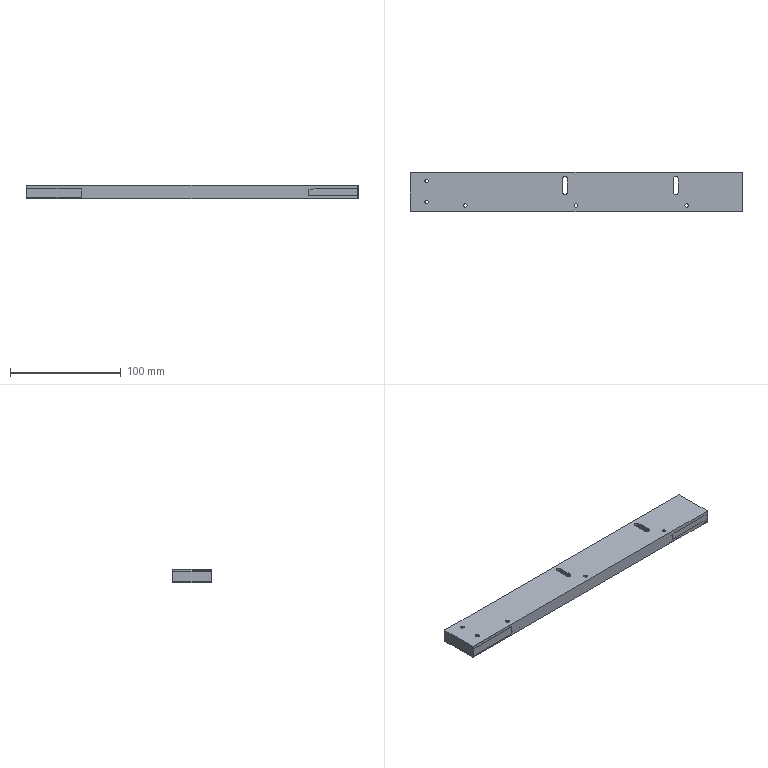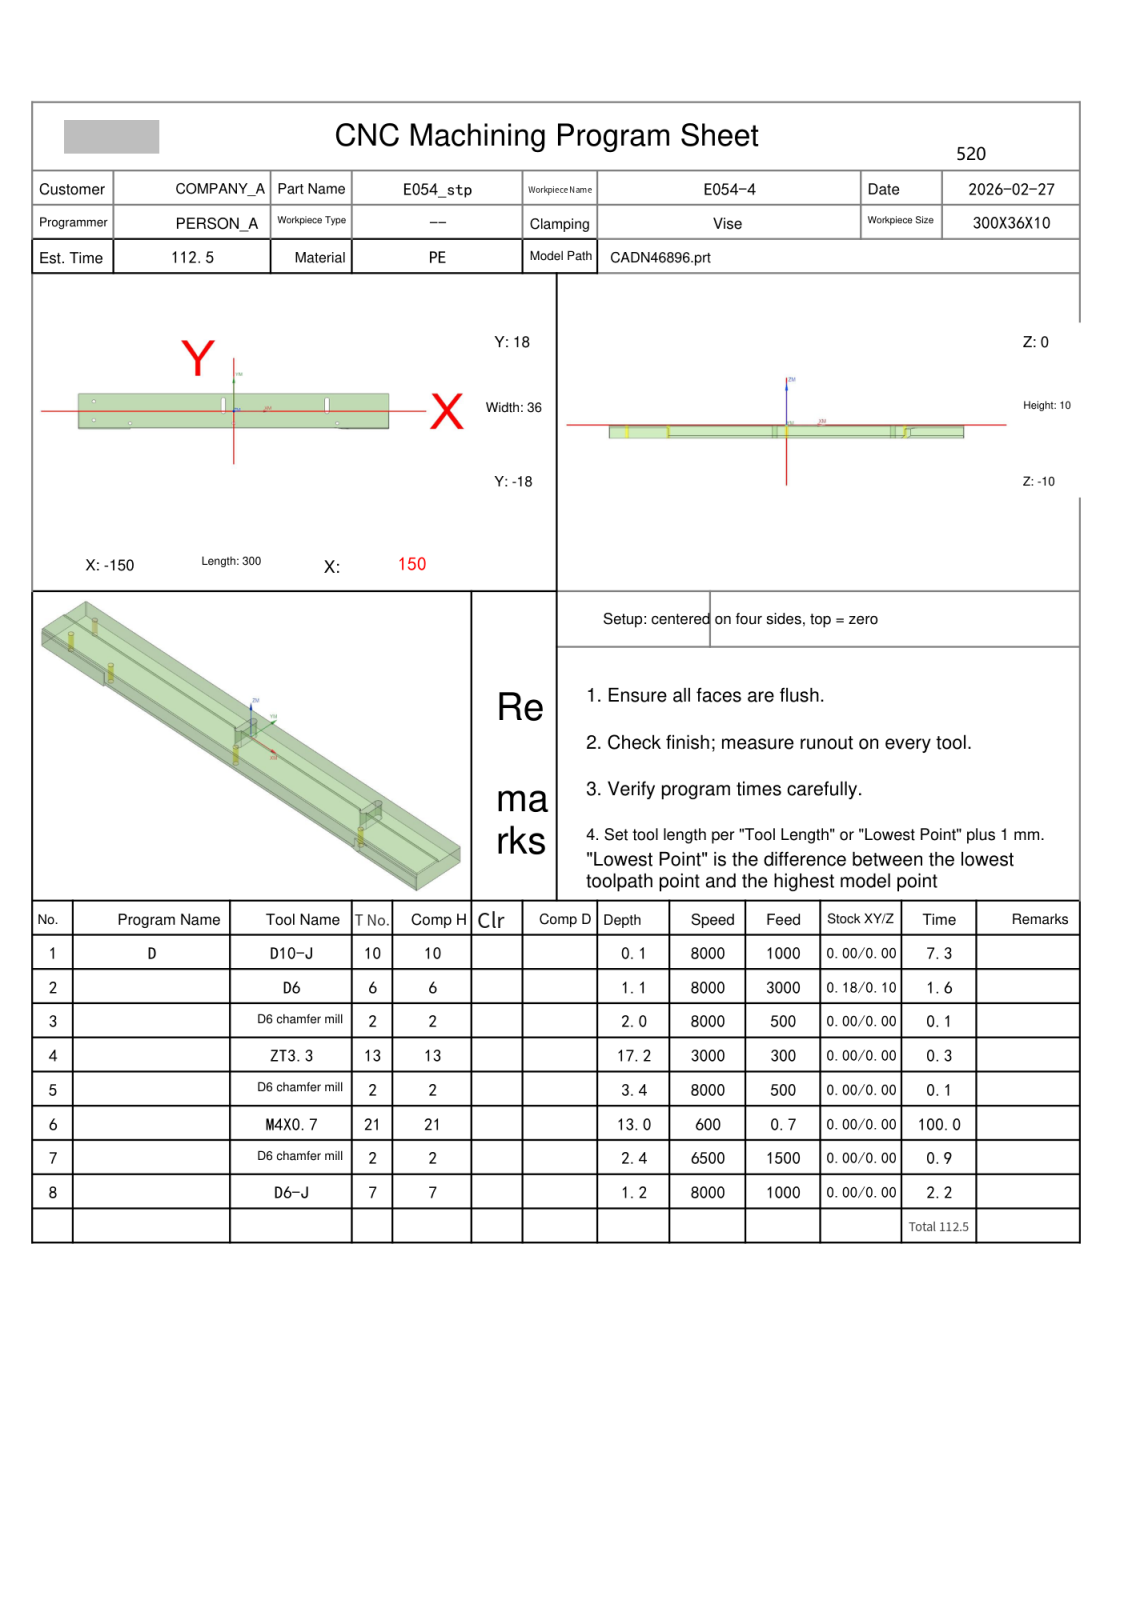NC program | NX | posted by the shop | part box 300 x 36 x 12 mm
Whole program:
%
O0001
(Machine time: 206.88 MIN)
(===Total Tool:6===)
(T10=D10-J  D=10.  R=0.   D-  H10 Z=0.    )
(T6=D6      D=6.   R=0.   D-  H06 Z=-1.1  )
(T2=D6 chamfer mill   D=6.   R=0.   D-  H02 Z=-3.37 )
(T13=ZT3.3  D=3.3  DR_a=118 D-  H13 Z=-17.2 )
(T21=M4X0.7 D=3.3  DR_a=180 D-  H21 Z=-13.  )
(T7=D6-J    D=6.   R=0.   D7  H07 Z=-1.2  )
G80 G90 G17 G49 G40
G91 G28 Z0
M01
N1 T10 M06
(D10-J  D=10. R=0. H=10 ce=0.00 di=0.10)
G00 G90 G54 X133.111 Y35. M03 S8000
G43 H10 Z50.
M08
Z2.55
G01 Z.55 F1000.
X145.111 Y23.
X155. Y13.111
Y3.222
X135.222 Y23.
X125.333
X155. Y-6.667
Y-16.556
X115.444 Y23.
X105.556
X151.556 Y-23.
X141.667
X95.667 Y23.
X85.778
X131.778 Y-23.
X121.889
X75.889 Y23.
X66.
X112. Y-23.
X102.111
X56.111 Y23.
X46.222
X92.222 Y-23.
X82.333
X36.333 Y23.
X26.444
X72.444 Y-23.
X62.556
X16.556 Y23.
X6.667
X52.667 Y-23.
X42.778
X-3.222 Y23.
X-13.111
X32.889 Y-23.
X23.
X-23. Y23.
X-32.889
X13.111 Y-23.
X3.222
X-42.778 Y23.
X-52.667
X-6.667 Y-23.
X-16.556
X-62.556 Y23.
X-72.444
X-26.444 Y-23.
X-36.333
X-82.333 Y23.
X-92.222
X-46.222 Y-23.
X-56.111
X-102.111 Y23.
X-112.
X-66. Y-23.
X-75.889
X-121.889 Y23.
X-131.778
X-85.778 Y-23.
X-95.667
X-141.667 Y23.
X-151.556
X-105.556 Y-23.
X-115.444
X-155. Y16.556
Y6.667
X-125.333 Y-23.
X-135.222
X-155. Y-3.222
Y-13.111
X-145.111 Y-23.
X-133.111 Y-35.
Z2.55
G00 Z4.
X167. Y1.111
Z2.1
G01 Z.1
X155. Y13.111
X145.111 Y23.
X135.222
X155. Y3.222
Y-6.667
X125.333 Y23.
X115.444
X155. Y-16.556
Y-23.
X151.556
X105.556 Y23.
X95.667
X141.667 Y-23.
X131.778
X85.778 Y23.
X75.889
X121.889 Y-23.
X112.
X66. Y23.
X56.111
X102.111 Y-23.
X92.222
X46.222 Y23.
X36.333
X82.333 Y-23.
X72.444
X26.444 Y23.
X16.556
X62.556 Y-23.
X52.667
X6.667 Y23.
X-3.222
X42.778 Y-23.
X32.889
X-13.111 Y23.
X-23.
X23. Y-23.
X13.111
X-32.889 Y23.
X-42.778
X3.222 Y-23.
X-6.667
X-52.667 Y23.
X-62.556
X-16.556 Y-23.
X-26.444
X-72.444 Y23.
X-82.333
X-36.333 Y-23.
X-46.222
X-92.222 Y23.
X-102.111
X-56.111 Y-23.
X-66.
X-112. Y23.
X-121.889
X-75.889 Y-23.
X-85.778
X-131.778 Y23.
X-141.667
X-95.667 Y-23.
X-105.556
X-151.556 Y23.
X-155.
Y16.556
X-115.444 Y-23.
X-125.333
X-155. Y6.667
Y-3.222
X-135.222 Y-23.
X-145.111
X-155. Y-13.111
X-167. Y-1.111
Z2.1
G00 Z50.
G00 G90 X133.111 Y35. M03 S8000
Z50.
Z2.
G01 Z0.0 F1000.
X145.111 Y23.
X155. Y13.111
Y3.222
X135.222 Y23.
X125.333
X155. Y-6.667
Y-16.556
X115.444 Y23.
X105.556
X151.556 Y-23.
X141.667
X95.667 Y23.
X85.778
X131.778 Y-23.
X121.889
X75.889 Y23.
X66.
X112. Y-23.
X102.111
X56.111 Y23.
X46.222
X92.222 Y-23.
X82.333
X36.333 Y23.
X26.444
X72.444 Y-23.
X62.556
X16.556 Y23.
X6.667
X52.667 Y-23.
X42.778
X-3.222 Y23.
X-13.111
X32.889 Y-23.
X23.
X-23. Y23.
X-32.889
X13.111 Y-23.
X3.222
X-42.778 Y23.
X-52.667
X-6.667 Y-23.
X-16.556
X-62.556 Y23.
X-72.444
X-26.444 Y-23.
X-36.333
X-82.333 Y23.
X-92.222
X-46.222 Y-23.
X-56.111
X-102.111 Y23.
X-112.
X-66. Y-23.
X-75.889
X-121.889 Y23.
X-131.778
X-85.778 Y-23.
X-95.667
X-141.667 Y23.
X-151.556
X-105.556 Y-23.
X-115.444
X-155. Y16.556
Y6.667
X-125.333 Y-23.
X-135.222
X-155. Y-3.222
Y-13.111
X-145.111 Y-23.
X-133.111 Y-35.
Z2.
G00 Z50.
G91 G28 Z0.0
M05
M09
G91 G28 Z0.0
M01
N2 T06 M06
(D6  D=6. R=0. H=06 ce=0.18 di=0.10)
G00 G90 G54 X-155.845 Y19.68 M03 S8000
G43 H06 Z11.
M08
Z1.133
G01 Z-.367 F3000.
X-151.978
X151.73
G02 X152.153 Y19.505 I-.001 J-.6
G01 X152.764 Y18.893
G02 X152.94 Y18.469 I-.424 J-.424
G01 Y17.279
G02 X152.341 Y16.68 I-.6 J.001
G01 X-152.341
G03 X-152.94 Y16.081 I.001 J-.6
G01 Y12.779
G03 X-152.341 Y12.18 I.6 J.001
G01 X152.341
G02 X152.94 Y11.581 I-.001 J-.6
G01 Y8.279
G02 X152.341 Y7.68 I-.6 J.001
G01 X-152.427
G03 X-153.019 Y7.173 I.001 J-.6
G01 X-153.533 Y3.872
X-153.54 Y3.78
G03 X-152.94 Y3.18 I.6 J0.0
G01 X152.94
X156.047
Z1.133
G00 X-155.845 Y19.68
Z.767
G01 Z-.733
X-151.978
X151.73
G02 X152.153 Y19.505 I-.001 J-.6
G01 X152.764 Y18.893
G02 X152.94 Y18.469 I-.424 J-.424
G01 Y17.279
G02 X152.341 Y16.68 I-.6 J.001
G01 X-152.341
G03 X-152.94 Y16.081 I.001 J-.6
G01 Y12.779
G03 X-152.341 Y12.18 I.6 J.001
G01 X152.341
G02 X152.94 Y11.581 I-.001 J-.6
G01 Y8.279
G02 X152.341 Y7.68 I-.6 J.001
G01 X-152.427
G03 X-153.019 Y7.173 I.001 J-.6
G01 X-153.533 Y3.872
X-153.54 Y3.78
G03 X-152.94 Y3.18 I.6 J0.0
G01 X152.94
X156.18
Z.767
G00 X-155.845 Y19.68
Z.4
G01 Z-1.1
X-151.978
X151.73
G02 X152.153 Y19.505 I-.001 J-.6
G01 X152.764 Y18.893
G02 X152.94 Y18.469 I-.424 J-.424
G01 Y17.279
G02 X152.341 Y16.68 I-.6 J.001
G01 X-152.341
G03 X-152.94 Y16.081 I.001 J-.6
G01 Y12.779
G03 X-152.341 Y12.18 I.6 J.001
G01 X152.341
G02 X152.94 Y11.581 I-.001 J-.6
G01 Y8.279
G02 X152.341 Y7.68 I-.6 J.001
G01 X-152.427
G03 X-153.019 Y7.173 I.001 J-.6
G01 X-153.533 Y3.872
X-153.54 Y3.78
G03 X-152.94 Y3.18 I.6 J0.0
G01 X152.94
X156.18
Z.4
G00 Z11.
G91 G28 Z0.0
M05
M09
G91 G28 Z0.0
M01
N3 T02 M06
(D6 chamfer mill  D=6. R=0. H=02 ce=0.00 di=0.10)
G00 G90 G54 X100. Y-12.2 M03 S8000
G43 H02 Z50.
M08
G98 G81 X100. Y-12.2 Z-.8 R1. F500.
X0.0
X-100.
X-135. Y-9.
Y10. Z-2. R-.2
G80
G00 Z50.
G91 G28 Z0.0
M05
M09
G91 G28 Z0.0
M01
N4 T13 M06
(ZT3.3 D=3.3 DR_a=118 H=13)
G00 G90 G54 X100. Y-12.2 M03 S3000
G43 H13 Z50.
M08
G98 G83 X100. Y-12.2 Z-16. R1. F300. Q2.
X0.0
X-100.
X-135. Y-9.
Y10. Z-17.2 R-.2
G80
G00 Z50.
G91 G28 Z0.0
M05
M09
G91 G28 Z0.0
M01
N5 T02 M06
(D6 chamfer mill  D=6. R=0. H=02 ce=0.00 di=0.10)
G00 G90 G54 X100. Y-12.2 M03 S8000
G43 H02 Z50.
M08
G98 G81 X100. Y-12.2 Z-2.171 R3. F500.
X0.0
X-100.
X-135. Y-9.
Y10. Z-3.371 R1.8
G80
G00 Z50.
G91 G28 Z0.0
M05
M09
G91 G28 Z0.0
M01
N6 T21 M06
(M4X0.7 D=3.3 DR_a=180 H=21)
G00 G90 G54 X100. Y-12.2 M03 S600
G43 H21 Z50.
M08
G95
G98 G84 X100. Y-12.2 Z-13. R1. F.7 Q4.
X0.0
X-100.
X-135. Y-9.
Y10.
G80
G94
G00 Z50.
G91 G28 Z0.0
M05
M09
G91 G28 Z0.0
M01
N7 T02 M06
(D6 chamfer mill  D=6. R=0. H=02 ce=0.00 di=0.00)
G00 G90 G54 X151.9 Y3.963 M03 S6500
G43 H02 Z50.
M08
Z.3
G01 Z-1.2 F1500.
G03 X150.7 Y2.763 I0.0 J-1.2
G01 Y-17.9
X-150.7
Y2.763
G03 X-151.9 Y3.963 I-1.2 J0.0
G01 Z.3
G00 Z50.
G00 G90 X-150.292 Y.99 M03 S6500
Z50.
Z.13
G01 Z-1.2 F1500.
G03 X-149.952 Y.915 I.601 J1.907
G01 X-149.898 Y.905
X-149.849 Y.928
X-149.759 Y.966
X-149.5 Y1.
X-12.25
G02 X-11.25 Y0.0 I0.0 J-1.
G01 Y-.2
G03 X-10. Y-1.45 I1.25 J0.0
X-8.75 Y-.2 I0.0 J1.25
G01 Y0.0
G02 X-7.75 Y1. I1. J0.0
G01 X87.75
G02 X88.75 Y0.0 I0.0 J-1.
G01 Y-.2
G03 X90. Y-1.45 I1.25 J0.0
X91.25 Y-.2 I0.0 J1.25
G01 Y0.0
G02 X92.25 Y1. I1. J0.0
G01 X149.5
X149.759 Y.966
X149.849 Y.928
X149.898 Y.905
X149.952 Y.915
G03 X150.292 Y.99 I-.261 J1.983
G01 Z.13
G00 Z10.
X100.465 Y-12.619
Z.411
G01 Z-1.2
G03 X100.612 Y-12.303 I-1.732 J1.
G01 X100.633 Y-12.253
X100.621 Y-12.2
G03 X100. Y-11.579 I-.621 J0.0
X99.379 Y-12.2 I0.0 J-.621
X100. Y-12.821 I.621 J0.0
X100.621 Y-12.2 I0.0 J.621
G01 X100.633 Y-12.147
X100.612 Y-12.097
G03 X100.465 Y-11.781 I-1.879 J-.684
G01 Z.411
G00 Z10.
X.465 Y-12.619
Z.411
G01 Z-1.2
G03 X.612 Y-12.303 I-1.732 J1.
G01 X.633 Y-12.253
X.621 Y-12.2
G03 X0.0 Y-11.579 I-.621 J0.0
X-.621 Y-12.2 I0.0 J-.621
X0.0 Y-12.821 I.621 J0.0
X.621 Y-12.2 I0.0 J.621
G01 X.633 Y-12.147
X.612 Y-12.097
G03 X.465 Y-11.781 I-1.879 J-.684
G01 Z.411
G00 Z10.
X-99.535 Y-12.619
Z.411
G01 Z-1.2
G03 X-99.388 Y-12.303 I-1.732 J1.
G01 X-99.367 Y-12.253
X-99.379 Y-12.2
G03 X-100. Y-11.579 I-.621 J0.0
X-100.621 Y-12.2 I0.0 J-.621
X-100. Y-12.821 I.621 J0.0
X-99.379 Y-12.2 I0.0 J.621
G01 X-99.367 Y-12.147
X-99.388 Y-12.097
G03 X-99.535 Y-11.781 I-1.879 J-.684
G01 Z.411
G00 Z10.
X-134.535 Y-9.419
Z.411
G01 Z-1.2
G03 X-134.388 Y-9.103 I-1.732 J1.
G01 X-134.367 Y-9.053
X-134.379 Y-9.
G03 X-135. Y-8.379 I-.621 J0.0
X-135.621 Y-9. I0.0 J-.621
X-135. Y-9.621 I.621 J0.0
X-134.379 Y-9. I0.0 J.621
G01 X-134.367 Y-8.947
X-134.388 Y-8.897
G03 X-134.535 Y-8.581 I-1.879 J-.684
G01 Z.411
G00 Z10.
X-8.75 Y2.166
Z1.6
G01 Z-2.4
Y11.8
G03 X-10. Y13.05 I-1.25 J0.0
X-11.25 Y11.8 I0.0 J-1.25
G01 Y2.166
Z1.6
G00 Z10.
X91.25
Z1.6
G01 Z-2.4
Y11.8
G03 X90. Y13.05 I-1.25 J0.0
X88.75 Y11.8 I0.0 J-1.25
G01 Y2.166
Z1.6
G00 Z10.
X-151. Y1.846
Z1.6
G01 Z-2.4
Y17.5
X-150.966 Y17.759
X-150.866 Y18.
X-150.707 Y18.207
X-150.207 Y18.707
X-150. Y18.866
X-149.759 Y18.966
X-149.5 Y19.
X149.5
X149.759 Y18.966
X150. Y18.866
X150.207 Y18.707
X150.707 Y18.207
X150.866 Y18.
X150.966 Y17.759
X151. Y17.5
Y1.846
Z1.6
G00 Z10.
X-135.465 Y10.419
Z-.787
G01 Z-2.4
G03 X-135.612 Y10.103 I1.732 J-1.
G01 X-135.633 Y10.053
X-135.621 Y10.
G03 X-135. Y9.379 I.621 J0.0
X-134.379 Y10. I0.0 J.621
X-135. Y10.621 I-.621 J0.0
X-135.621 Y10. I0.0 J-.621
G01 X-135.633 Y9.947
X-135.612 Y9.897
G03 X-135.465 Y9.581 I1.879 J.684
G01 Z-.787
G00 Z50.
G91 G28 Z0.0
M05
M09
G91 G28 Z0.0
M01
N8 T07 M06
(D6-J  D=6. R=0. H=07 ce=0.40 di=0.00)
G00 G90 G54 X-1.2 Y22.2 M03 S8000
G43 H07 Z11.
M08
Z.3
G01 Z-1.2 F1000.
Y19.8
G03 X0.0 Y18.6 I1.2 J0.0
G01 X149.504
G02 X149.922 Y18.427 I-.004 J-.6
G01 X150.427 Y17.922
G02 X150.6 Y17.504 I-.427 J-.422
G01 Y3.996
G02 X150.004 Y3.4 I-.6 J.004
G01 X-150.004
G02 X-150.6 Y3.996 I.004 J.6
G01 Y17.504
G02 X-150.427 Y17.922 I.6 J-.004
G01 X-149.922 Y18.427
G02 X-149.504 Y18.6 I.422 J-.427
G01 X1.252
G02 X1.675 Y18.425 I-.001 J-.6
G01 X4.325 Y15.775
G03 X4.748 Y15.6 I.424 J.425
G01 X147.004
G02 X147.6 Y15.004 I-.004 J-.6
G01 Y6.996
G02 X147.004 Y6.4 I-.6 J.004
G01 X-147.004
G02 X-147.6 Y6.996 I.004 J.6
G01 Y15.004
G02 X-147.004 Y15.6 I.6 J-.004
G01 X1.252
G02 X1.675 Y15.425 I-.001 J-.6
G01 X4.325 Y12.775
G03 X4.748 Y12.6 I.424 J.425
G01 X144.004
G02 X144.6 Y12.004 I-.004 J-.6
G01 Y9.996
G02 X144.004 Y9.4 I-.6 J.004
G01 X-144.004
G02 X-144.6 Y9.996 I.004 J.6
G01 Y12.004
G02 X-144.004 Y12.6 I.6 J-.004
G01 X3.
X4.
G03 X5.2 Y13.8 I0.0 J1.2
G01 Z.3
G00 Z11.
G00 G90 X-154.2 Y4.399 M03 S8000
Z11.
Z-.2
G01 Z-1.2 F1000.
G41 D07
Y4.199
G03 X-153. Y3. I1.2 J.001
G01 X153.
G03 X154.2 Y4.199 I0.0 J1.2
G01 G40 Y4.399
Z-.2
G00 Z11.
M05
M09
G91 G28 Z0.0
G91 G28 Y0.0
M30
%